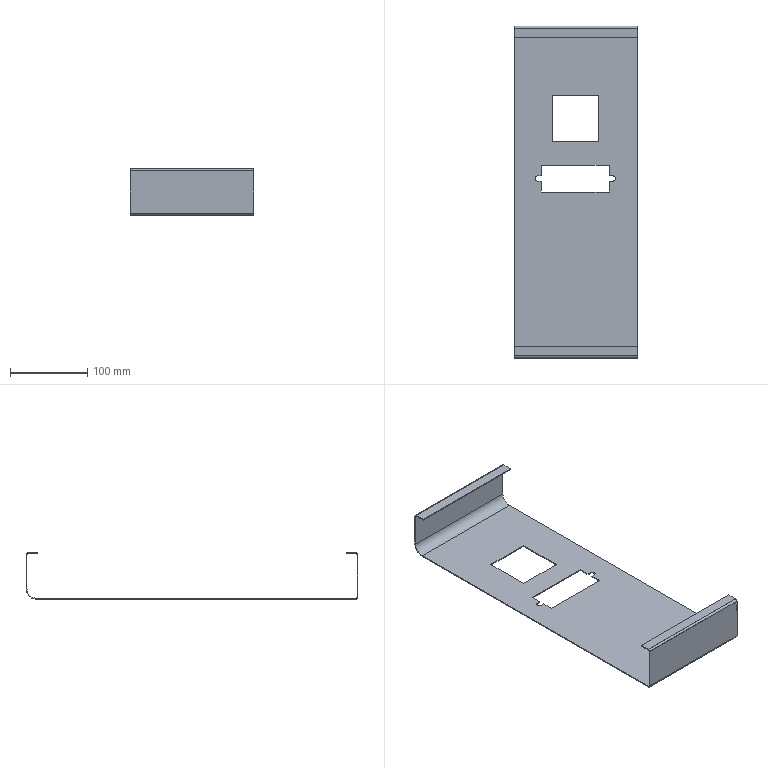Part | SolidWorks | features FlatPattern 1, ICE 1, SMBaseFlange 1, SheetMetal 1 | 1 solid | 55 faces | box 160 x 430 x 60 mm | volume 100743 mm3 | plane 44 | cylinder 11 | commonest cylinder face diameters 3 x3 5.4 x3 7 x3 24 x1 26.4 x1
STEP:
#1=CARTESIAN_POINT('',(-49.5,21.,1.2));
#2=VERTEX_POINT('',#1);
#3=CARTESIAN_POINT('',(-53.,17.5,1.2));
#4=VERTEX_POINT('',#3);
#5=CARTESIAN_POINT('',(-49.5,17.5,1.2));
#6=DIRECTION('',(0.,0.,1.));
#7=DIRECTION('',(0.,1.,0.));
#8=AXIS2_PLACEMENT_3D('',#5,#6,#7);
#9=CIRCLE('',#8,3.5);
#10=EDGE_CURVE('',#2,#4,#9,.T.);
#11=ORIENTED_EDGE('',*,*,#10,.T.);
#12=CARTESIAN_POINT('',(-53.,17.5,0.));
#13=VERTEX_POINT('',#12);
#14=CARTESIAN_POINT('',(-53.,17.5,60.001));
#15=DIRECTION('',(0.,0.,-1.));
#16=VECTOR('',#15,1000.);
#17=LINE('',#14,#16);
#18=EDGE_CURVE('',#4,#13,#17,.T.);
#19=ORIENTED_EDGE('',*,*,#18,.T.);
#20=CARTESIAN_POINT('',(-49.5,21.,0.));
#21=VERTEX_POINT('',#20);
#22=CARTESIAN_POINT('',(-49.5,17.5,0.));
#23=DIRECTION('',(0.,0.,-1.));
#24=DIRECTION('',(-1.,0.,0.));
#25=AXIS2_PLACEMENT_3D('',#22,#23,#24);
#26=CIRCLE('',#25,3.5);
#27=EDGE_CURVE('',#13,#21,#26,.T.);
#28=ORIENTED_EDGE('',*,*,#27,.T.);
#29=CARTESIAN_POINT('',(-49.5,21.,60.001));
#30=DIRECTION('',(0.,0.,-1.));
#31=VECTOR('',#30,1000.);
#32=LINE('',#29,#31);
#33=EDGE_CURVE('',#2,#21,#32,.T.);
#34=ORIENTED_EDGE('',*,*,#33,.F.);
#35=EDGE_LOOP('',(#11,#19,#28,#34));
#36=FACE_OUTER_BOUND('',#35,.T.);
#37=CARTESIAN_POINT('',(-49.5,17.5,60.001));
#38=DIRECTION('',(0.,0.,-1.));
#39=DIRECTION('',(-1.,0.,0.));
#40=AXIS2_PLACEMENT_3D('',#37,#38,#39);
#41=CYLINDRICAL_SURFACE('',#40,3.5);
#42=ADVANCED_FACE('',(#36),#41,.F.);
#43=CARTESIAN_POINT('',(80.,201.8,0.));
#44=VERTEX_POINT('',#43);
#45=CARTESIAN_POINT('',(80.,201.8,1.2));
#46=VERTEX_POINT('',#45);
#47=CARTESIAN_POINT('',(80.,201.8,0.));
#48=DIRECTION('',(0.,0.,1.));
#49=VECTOR('',#48,1000.);
#50=LINE('',#47,#49);
#51=EDGE_CURVE('',#44,#46,#50,.T.);
#52=ORIENTED_EDGE('',*,*,#51,.F.);
#53=CARTESIAN_POINT('',(80.,215.,13.2));
#54=VERTEX_POINT('',#53);
#55=CARTESIAN_POINT('',(80.,201.8,13.2));
#56=DIRECTION('',(-1.,0.,0.));
#57=DIRECTION('',(0.,0.,-1.));
#58=AXIS2_PLACEMENT_3D('',#55,#56,#57);
#59=CIRCLE('',#58,13.2);
#60=EDGE_CURVE('',#54,#44,#59,.T.);
#61=ORIENTED_EDGE('',*,*,#60,.F.);
#62=CARTESIAN_POINT('',(80.,213.8,13.2));
#63=VERTEX_POINT('',#62);
#64=CARTESIAN_POINT('',(80.,213.8,13.2));
#65=DIRECTION('',(0.,1.,0.));
#66=VECTOR('',#65,1000.);
#67=LINE('',#64,#66);
#68=EDGE_CURVE('',#63,#54,#67,.T.);
#69=ORIENTED_EDGE('',*,*,#68,.F.);
#70=CARTESIAN_POINT('',(80.,201.8,13.2));
#71=DIRECTION('',(-1.,0.,0.));
#72=DIRECTION('',(0.,0.,-1.));
#73=AXIS2_PLACEMENT_3D('',#70,#71,#72);
#74=CIRCLE('',#73,12.);
#75=EDGE_CURVE('',#63,#46,#74,.T.);
#76=ORIENTED_EDGE('',*,*,#75,.T.);
#77=EDGE_LOOP('',(#52,#61,#69,#76));
#78=FACE_OUTER_BOUND('',#77,.T.);
#79=CARTESIAN_POINT('',(80.,201.8,0.));
#80=DIRECTION('',(1.,0.,0.));
#81=DIRECTION('',(0.,0.,-1.));
#82=AXIS2_PLACEMENT_3D('',#79,#80,#81);
#83=PLANE('',#82);
#84=ADVANCED_FACE('',(#78),#83,.T.);
#85=CARTESIAN_POINT('',(80.,-212.3,0.));
#86=VERTEX_POINT('',#85);
#87=CARTESIAN_POINT('',(80.,0.,0.));
#88=DIRECTION('',(0.,-1.,0.));
#89=VECTOR('',#88,1000.);
#90=LINE('',#87,#89);
#91=EDGE_CURVE('',#44,#86,#90,.T.);
#92=ORIENTED_EDGE('',*,*,#91,.F.);
#93=ORIENTED_EDGE('',*,*,#51,.T.);
#94=CARTESIAN_POINT('',(80.,-212.3,1.2));
#95=VERTEX_POINT('',#94);
#96=CARTESIAN_POINT('',(80.,0.,1.2));
#97=DIRECTION('',(0.,-1.,0.));
#98=VECTOR('',#97,1000.);
#99=LINE('',#96,#98);
#100=EDGE_CURVE('',#46,#95,#99,.T.);
#101=ORIENTED_EDGE('',*,*,#100,.T.);
#102=CARTESIAN_POINT('',(80.,-212.3,1.2));
#103=DIRECTION('',(0.,0.,-1.));
#104=VECTOR('',#103,1000.);
#105=LINE('',#102,#104);
#106=EDGE_CURVE('',#95,#86,#105,.T.);
#107=ORIENTED_EDGE('',*,*,#106,.T.);
#108=EDGE_LOOP('',(#92,#93,#101,#107));
#109=FACE_OUTER_BOUND('',#108,.T.);
#110=CARTESIAN_POINT('',(80.,213.8,13.2));
#111=DIRECTION('',(1.,0.,0.));
#112=DIRECTION('',(0.,0.,-1.));
#113=AXIS2_PLACEMENT_3D('',#110,#111,#112);
#114=PLANE('',#113);
#115=ADVANCED_FACE('',(#109),#114,.T.);
#116=CARTESIAN_POINT('',(-80.,215.,13.2));
#117=VERTEX_POINT('',#116);
#118=CARTESIAN_POINT('',(-80.,213.8,13.2));
#119=VERTEX_POINT('',#118);
#120=CARTESIAN_POINT('',(-80.,215.,13.2));
#121=DIRECTION('',(0.,-1.,0.));
#122=VECTOR('',#121,1000.);
#123=LINE('',#120,#122);
#124=EDGE_CURVE('',#117,#119,#123,.T.);
#125=ORIENTED_EDGE('',*,*,#124,.F.);
#126=CARTESIAN_POINT('',(-80.,201.8,0.));
#127=VERTEX_POINT('',#126);
#128=CARTESIAN_POINT('',(-80.,201.8,13.2));
#129=DIRECTION('',(-1.,0.,0.));
#130=DIRECTION('',(0.,0.,-1.));
#131=AXIS2_PLACEMENT_3D('',#128,#129,#130);
#132=CIRCLE('',#131,13.2);
#133=EDGE_CURVE('',#117,#127,#132,.T.);
#134=ORIENTED_EDGE('',*,*,#133,.T.);
#135=CARTESIAN_POINT('',(-80.,201.8,1.2));
#136=VERTEX_POINT('',#135);
#137=CARTESIAN_POINT('',(-80.,201.8,1.2));
#138=DIRECTION('',(0.,0.,-1.));
#139=VECTOR('',#138,1000.);
#140=LINE('',#137,#139);
#141=EDGE_CURVE('',#136,#127,#140,.T.);
#142=ORIENTED_EDGE('',*,*,#141,.F.);
#143=CARTESIAN_POINT('',(-80.,201.8,13.2));
#144=DIRECTION('',(-1.,0.,0.));
#145=DIRECTION('',(0.,0.,-1.));
#146=AXIS2_PLACEMENT_3D('',#143,#144,#145);
#147=CIRCLE('',#146,12.);
#148=EDGE_CURVE('',#119,#136,#147,.T.);
#149=ORIENTED_EDGE('',*,*,#148,.F.);
#150=EDGE_LOOP('',(#125,#134,#142,#149));
#151=FACE_OUTER_BOUND('',#150,.T.);
#152=CARTESIAN_POINT('',(-80.,215.,13.2));
#153=DIRECTION('',(-1.,0.,0.));
#154=DIRECTION('',(0.,0.,1.));
#155=AXIS2_PLACEMENT_3D('',#152,#153,#154);
#156=PLANE('',#155);
#157=ADVANCED_FACE('',(#151),#156,.T.);
#158=CARTESIAN_POINT('',(-80.,215.,57.3));
#159=VERTEX_POINT('',#158);
#160=CARTESIAN_POINT('',(-80.,215.,13.2));
#161=DIRECTION('',(0.,0.,-1.));
#162=VECTOR('',#161,1000.);
#163=LINE('',#160,#162);
#164=EDGE_CURVE('',#159,#117,#163,.T.);
#165=ORIENTED_EDGE('',*,*,#164,.T.);
#166=ORIENTED_EDGE('',*,*,#124,.T.);
#167=CARTESIAN_POINT('',(-80.,213.8,57.3));
#168=VERTEX_POINT('',#167);
#169=CARTESIAN_POINT('',(-80.,213.8,13.2));
#170=DIRECTION('',(0.,0.,-1.));
#171=VECTOR('',#170,1000.);
#172=LINE('',#169,#171);
#173=EDGE_CURVE('',#168,#119,#172,.T.);
#174=ORIENTED_EDGE('',*,*,#173,.F.);
#175=CARTESIAN_POINT('',(-80.,213.8,57.3));
#176=DIRECTION('',(0.,1.,0.));
#177=VECTOR('',#176,1000.);
#178=LINE('',#175,#177);
#179=EDGE_CURVE('',#168,#159,#178,.T.);
#180=ORIENTED_EDGE('',*,*,#179,.T.);
#181=EDGE_LOOP('',(#165,#166,#174,#180));
#182=FACE_OUTER_BOUND('',#181,.T.);
#183=CARTESIAN_POINT('',(-80.,201.8,1.2));
#184=DIRECTION('',(-1.,0.,0.));
#185=DIRECTION('',(0.,0.,1.));
#186=AXIS2_PLACEMENT_3D('',#183,#184,#185);
#187=PLANE('',#186);
#188=ADVANCED_FACE('',(#182),#187,.T.);
#189=CARTESIAN_POINT('',(80.,215.,57.3));
#190=VERTEX_POINT('',#189);
#191=CARTESIAN_POINT('',(80.,213.8,57.3));
#192=VERTEX_POINT('',#191);
#193=CARTESIAN_POINT('',(80.,215.,57.3));
#194=DIRECTION('',(0.,-1.,0.));
#195=VECTOR('',#194,1000.);
#196=LINE('',#193,#195);
#197=EDGE_CURVE('',#190,#192,#196,.T.);
#198=ORIENTED_EDGE('',*,*,#197,.F.);
#199=CARTESIAN_POINT('',(80.,212.3,60.));
#200=VERTEX_POINT('',#199);
#201=CARTESIAN_POINT('',(80.,212.3,57.3));
#202=DIRECTION('',(-1.,0.,0.));
#203=DIRECTION('',(0.,0.,-1.));
#204=AXIS2_PLACEMENT_3D('',#201,#202,#203);
#205=CIRCLE('',#204,2.7);
#206=EDGE_CURVE('',#200,#190,#205,.T.);
#207=ORIENTED_EDGE('',*,*,#206,.F.);
#208=CARTESIAN_POINT('',(80.,212.3,58.8));
#209=VERTEX_POINT('',#208);
#210=CARTESIAN_POINT('',(80.,212.3,58.8));
#211=DIRECTION('',(0.,0.,1.));
#212=VECTOR('',#211,1000.);
#213=LINE('',#210,#212);
#214=EDGE_CURVE('',#209,#200,#213,.T.);
#215=ORIENTED_EDGE('',*,*,#214,.F.);
#216=CARTESIAN_POINT('',(80.,212.3,57.3));
#217=DIRECTION('',(-1.,0.,0.));
#218=DIRECTION('',(0.,0.,-1.));
#219=AXIS2_PLACEMENT_3D('',#216,#217,#218);
#220=CIRCLE('',#219,1.5);
#221=EDGE_CURVE('',#209,#192,#220,.T.);
#222=ORIENTED_EDGE('',*,*,#221,.T.);
#223=EDGE_LOOP('',(#198,#207,#215,#222));
#224=FACE_OUTER_BOUND('',#223,.T.);
#225=CARTESIAN_POINT('',(80.,215.,57.3));
#226=DIRECTION('',(1.,0.,0.));
#227=DIRECTION('',(0.,0.,-1.));
#228=AXIS2_PLACEMENT_3D('',#225,#226,#227);
#229=PLANE('',#228);
#230=ADVANCED_FACE('',(#224),#229,.T.);
#231=CARTESIAN_POINT('',(80.,215.,13.2));
#232=DIRECTION('',(0.,0.,-1.));
#233=VECTOR('',#232,1000.);
#234=LINE('',#231,#233);
#235=EDGE_CURVE('',#190,#54,#234,.T.);
#236=ORIENTED_EDGE('',*,*,#235,.F.);
#237=ORIENTED_EDGE('',*,*,#197,.T.);
#238=CARTESIAN_POINT('',(80.,213.8,13.2));
#239=DIRECTION('',(0.,0.,-1.));
#240=VECTOR('',#239,1000.);
#241=LINE('',#238,#240);
#242=EDGE_CURVE('',#192,#63,#241,.T.);
#243=ORIENTED_EDGE('',*,*,#242,.T.);
#244=ORIENTED_EDGE('',*,*,#68,.T.);
#245=EDGE_LOOP('',(#236,#237,#243,#244));
#246=FACE_OUTER_BOUND('',#245,.T.);
#247=CARTESIAN_POINT('',(80.,212.3,58.8));
#248=DIRECTION('',(1.,0.,0.));
#249=DIRECTION('',(0.,0.,-1.));
#250=AXIS2_PLACEMENT_3D('',#247,#248,#249);
#251=PLANE('',#250);
#252=ADVANCED_FACE('',(#246),#251,.T.);
#253=CARTESIAN_POINT('',(-80.,212.3,60.));
#254=VERTEX_POINT('',#253);
#255=CARTESIAN_POINT('',(-80.,212.3,58.8));
#256=VERTEX_POINT('',#255);
#257=CARTESIAN_POINT('',(-80.,212.3,60.));
#258=DIRECTION('',(0.,0.,-1.));
#259=VECTOR('',#258,1000.);
#260=LINE('',#257,#259);
#261=EDGE_CURVE('',#254,#256,#260,.T.);
#262=ORIENTED_EDGE('',*,*,#261,.F.);
#263=CARTESIAN_POINT('',(-80.,212.3,57.3));
#264=DIRECTION('',(-1.,0.,0.));
#265=DIRECTION('',(0.,0.,-1.));
#266=AXIS2_PLACEMENT_3D('',#263,#264,#265);
#267=CIRCLE('',#266,2.7);
#268=EDGE_CURVE('',#254,#159,#267,.T.);
#269=ORIENTED_EDGE('',*,*,#268,.T.);
#270=ORIENTED_EDGE('',*,*,#179,.F.);
#271=CARTESIAN_POINT('',(-80.,212.3,57.3));
#272=DIRECTION('',(-1.,0.,0.));
#273=DIRECTION('',(0.,0.,-1.));
#274=AXIS2_PLACEMENT_3D('',#271,#272,#273);
#275=CIRCLE('',#274,1.5);
#276=EDGE_CURVE('',#256,#168,#275,.T.);
#277=ORIENTED_EDGE('',*,*,#276,.F.);
#278=EDGE_LOOP('',(#262,#269,#270,#277));
#279=FACE_OUTER_BOUND('',#278,.T.);
#280=CARTESIAN_POINT('',(-80.,212.3,60.));
#281=DIRECTION('',(-1.,0.,0.));
#282=DIRECTION('',(0.,0.,1.));
#283=AXIS2_PLACEMENT_3D('',#280,#281,#282);
#284=PLANE('',#283);
#285=ADVANCED_FACE('',(#279),#284,.T.);
#286=CARTESIAN_POINT('',(-80.,200.,60.));
#287=VERTEX_POINT('',#286);
#288=CARTESIAN_POINT('',(-80.,215.,60.));
#289=DIRECTION('',(0.,1.,0.));
#290=VECTOR('',#289,1000.);
#291=LINE('',#288,#290);
#292=EDGE_CURVE('',#287,#254,#291,.T.);
#293=ORIENTED_EDGE('',*,*,#292,.T.);
#294=ORIENTED_EDGE('',*,*,#261,.T.);
#295=CARTESIAN_POINT('',(-80.,200.,58.8));
#296=VERTEX_POINT('',#295);
#297=CARTESIAN_POINT('',(-80.,215.,58.8));
#298=DIRECTION('',(0.,1.,0.));
#299=VECTOR('',#298,1000.);
#300=LINE('',#297,#299);
#301=EDGE_CURVE('',#296,#256,#300,.T.);
#302=ORIENTED_EDGE('',*,*,#301,.F.);
#303=CARTESIAN_POINT('',(-80.,200.,58.8));
#304=DIRECTION('',(0.,0.,1.));
#305=VECTOR('',#304,1000.);
#306=LINE('',#303,#305);
#307=EDGE_CURVE('',#296,#287,#306,.T.);
#308=ORIENTED_EDGE('',*,*,#307,.T.);
#309=EDGE_LOOP('',(#293,#294,#302,#308));
#310=FACE_OUTER_BOUND('',#309,.T.);
#311=CARTESIAN_POINT('',(-80.,213.8,57.3));
#312=DIRECTION('',(-1.,0.,0.));
#313=DIRECTION('',(0.,0.,1.));
#314=AXIS2_PLACEMENT_3D('',#311,#312,#313);
#315=PLANE('',#314);
#316=ADVANCED_FACE('',(#310),#315,.T.);
#317=CARTESIAN_POINT('',(80.,-215.,2.7));
#318=VERTEX_POINT('',#317);
#319=CARTESIAN_POINT('',(80.,-213.8,2.7));
#320=VERTEX_POINT('',#319);
#321=CARTESIAN_POINT('',(80.,-215.,2.7));
#322=DIRECTION('',(0.,1.,0.));
#323=VECTOR('',#322,1000.);
#324=LINE('',#321,#323);
#325=EDGE_CURVE('',#318,#320,#324,.T.);
#326=ORIENTED_EDGE('',*,*,#325,.F.);
#327=CARTESIAN_POINT('',(80.,-212.3,2.7));
#328=DIRECTION('',(-1.,0.,0.));
#329=DIRECTION('',(0.,0.,-1.));
#330=AXIS2_PLACEMENT_3D('',#327,#328,#329);
#331=CIRCLE('',#330,2.7);
#332=EDGE_CURVE('',#86,#318,#331,.T.);
#333=ORIENTED_EDGE('',*,*,#332,.F.);
#334=ORIENTED_EDGE('',*,*,#106,.F.);
#335=CARTESIAN_POINT('',(80.,-212.3,2.7));
#336=DIRECTION('',(-1.,0.,0.));
#337=DIRECTION('',(0.,0.,-1.));
#338=AXIS2_PLACEMENT_3D('',#335,#336,#337);
#339=CIRCLE('',#338,1.5);
#340=EDGE_CURVE('',#95,#320,#339,.T.);
#341=ORIENTED_EDGE('',*,*,#340,.T.);
#342=EDGE_LOOP('',(#326,#333,#334,#341));
#343=FACE_OUTER_BOUND('',#342,.T.);
#344=CARTESIAN_POINT('',(80.,-215.,2.7));
#345=DIRECTION('',(1.,0.,0.));
#346=DIRECTION('',(0.,0.,-1.));
#347=AXIS2_PLACEMENT_3D('',#344,#345,#346);
#348=PLANE('',#347);
#349=ADVANCED_FACE('',(#343),#348,.T.);
#350=CARTESIAN_POINT('',(80.,-215.,57.3));
#351=VERTEX_POINT('',#350);
#352=CARTESIAN_POINT('',(80.,-215.,0.));
#353=DIRECTION('',(0.,0.,1.));
#354=VECTOR('',#353,1000.);
#355=LINE('',#352,#354);
#356=EDGE_CURVE('',#318,#351,#355,.T.);
#357=ORIENTED_EDGE('',*,*,#356,.F.);
#358=ORIENTED_EDGE('',*,*,#325,.T.);
#359=CARTESIAN_POINT('',(80.,-213.8,57.3));
#360=VERTEX_POINT('',#359);
#361=CARTESIAN_POINT('',(80.,-213.8,0.));
#362=DIRECTION('',(0.,0.,1.));
#363=VECTOR('',#362,1000.);
#364=LINE('',#361,#363);
#365=EDGE_CURVE('',#320,#360,#364,.T.);
#366=ORIENTED_EDGE('',*,*,#365,.T.);
#367=CARTESIAN_POINT('',(80.,-213.8,57.3));
#368=DIRECTION('',(0.,-1.,0.));
#369=VECTOR('',#368,1000.);
#370=LINE('',#367,#369);
#371=EDGE_CURVE('',#360,#351,#370,.T.);
#372=ORIENTED_EDGE('',*,*,#371,.T.);
#373=EDGE_LOOP('',(#357,#358,#366,#372));
#374=FACE_OUTER_BOUND('',#373,.T.);
#375=CARTESIAN_POINT('',(80.,-212.3,1.2));
#376=DIRECTION('',(1.,0.,0.));
#377=DIRECTION('',(0.,0.,-1.));
#378=AXIS2_PLACEMENT_3D('',#375,#376,#377);
#379=PLANE('',#378);
#380=ADVANCED_FACE('',(#374),#379,.T.);
#381=CARTESIAN_POINT('',(-80.,-212.3,0.));
#382=VERTEX_POINT('',#381);
#383=CARTESIAN_POINT('',(-80.,-212.3,1.2));
#384=VERTEX_POINT('',#383);
#385=CARTESIAN_POINT('',(-80.,-212.3,0.));
#386=DIRECTION('',(0.,0.,1.));
#387=VECTOR('',#386,1000.);
#388=LINE('',#385,#387);
#389=EDGE_CURVE('',#382,#384,#388,.T.);
#390=ORIENTED_EDGE('',*,*,#389,.F.);
#391=CARTESIAN_POINT('',(-80.,-215.,2.7));
#392=VERTEX_POINT('',#391);
#393=CARTESIAN_POINT('',(-80.,-212.3,2.7));
#394=DIRECTION('',(-1.,0.,0.));
#395=DIRECTION('',(0.,0.,-1.));
#396=AXIS2_PLACEMENT_3D('',#393,#394,#395);
#397=CIRCLE('',#396,2.7);
#398=EDGE_CURVE('',#382,#392,#397,.T.);
#399=ORIENTED_EDGE('',*,*,#398,.T.);
#400=CARTESIAN_POINT('',(-80.,-213.8,2.7));
#401=VERTEX_POINT('',#400);
#402=CARTESIAN_POINT('',(-80.,-213.8,2.7));
#403=DIRECTION('',(0.,-1.,0.));
#404=VECTOR('',#403,1000.);
#405=LINE('',#402,#404);
#406=EDGE_CURVE('',#401,#392,#405,.T.);
#407=ORIENTED_EDGE('',*,*,#406,.F.);
#408=CARTESIAN_POINT('',(-80.,-212.3,2.7));
#409=DIRECTION('',(-1.,0.,0.));
#410=DIRECTION('',(0.,0.,-1.));
#411=AXIS2_PLACEMENT_3D('',#408,#409,#410);
#412=CIRCLE('',#411,1.5);
#413=EDGE_CURVE('',#384,#401,#412,.T.);
#414=ORIENTED_EDGE('',*,*,#413,.F.);
#415=EDGE_LOOP('',(#390,#399,#407,#414));
#416=FACE_OUTER_BOUND('',#415,.T.);
#417=CARTESIAN_POINT('',(-80.,-212.3,0.));
#418=DIRECTION('',(-1.,0.,0.));
#419=DIRECTION('',(0.,0.,1.));
#420=AXIS2_PLACEMENT_3D('',#417,#418,#419);
#421=PLANE('',#420);
#422=ADVANCED_FACE('',(#416),#421,.T.);
#423=CARTESIAN_POINT('',(-80.,0.,0.));
#424=DIRECTION('',(0.,-1.,0.));
#425=VECTOR('',#424,1000.);
#426=LINE('',#423,#425);
#427=EDGE_CURVE('',#127,#382,#426,.T.);
#428=ORIENTED_EDGE('',*,*,#427,.T.);
#429=ORIENTED_EDGE('',*,*,#389,.T.);
#430=CARTESIAN_POINT('',(-80.,0.,1.2));
#431=DIRECTION('',(0.,-1.,0.));
#432=VECTOR('',#431,1000.);
#433=LINE('',#430,#432);
#434=EDGE_CURVE('',#136,#384,#433,.T.);
#435=ORIENTED_EDGE('',*,*,#434,.F.);
#436=ORIENTED_EDGE('',*,*,#141,.T.);
#437=EDGE_LOOP('',(#428,#429,#435,#436));
#438=FACE_OUTER_BOUND('',#437,.T.);
#439=CARTESIAN_POINT('',(-80.,-213.8,2.7));
#440=DIRECTION('',(-1.,0.,0.));
#441=DIRECTION('',(0.,0.,1.));
#442=AXIS2_PLACEMENT_3D('',#439,#440,#441);
#443=PLANE('',#442);
#444=ADVANCED_FACE('',(#438),#443,.T.);
#445=CARTESIAN_POINT('',(80.,-212.3,60.));
#446=VERTEX_POINT('',#445);
#447=CARTESIAN_POINT('',(80.,-212.3,58.8));
#448=VERTEX_POINT('',#447);
#449=CARTESIAN_POINT('',(80.,-212.3,60.));
#450=DIRECTION('',(0.,0.,-1.));
#451=VECTOR('',#450,1000.);
#452=LINE('',#449,#451);
#453=EDGE_CURVE('',#446,#448,#452,.T.);
#454=ORIENTED_EDGE('',*,*,#453,.F.);
#455=CARTESIAN_POINT('',(80.,-212.3,57.3));
#456=DIRECTION('',(-1.,0.,0.));
#457=DIRECTION('',(0.,0.,-1.));
#458=AXIS2_PLACEMENT_3D('',#455,#456,#457);
#459=CIRCLE('',#458,2.7);
#460=EDGE_CURVE('',#351,#446,#459,.T.);
#461=ORIENTED_EDGE('',*,*,#460,.F.);
#462=ORIENTED_EDGE('',*,*,#371,.F.);
#463=CARTESIAN_POINT('',(80.,-212.3,57.3));
#464=DIRECTION('',(-1.,0.,0.));
#465=DIRECTION('',(0.,0.,-1.));
#466=AXIS2_PLACEMENT_3D('',#463,#464,#465);
#467=CIRCLE('',#466,1.5);
#468=EDGE_CURVE('',#360,#448,#467,.T.);
#469=ORIENTED_EDGE('',*,*,#468,.T.);
#470=EDGE_LOOP('',(#454,#461,#462,#469));
#471=FACE_OUTER_BOUND('',#470,.T.);
#472=CARTESIAN_POINT('',(80.,-212.3,60.));
#473=DIRECTION('',(1.,0.,0.));
#474=DIRECTION('',(0.,0.,-1.));
#475=AXIS2_PLACEMENT_3D('',#472,#473,#474);
#476=PLANE('',#475);
#477=ADVANCED_FACE('',(#471),#476,.T.);
#478=CARTESIAN_POINT('',(80.,-200.,60.));
#479=VERTEX_POINT('',#478);
#480=CARTESIAN_POINT('',(80.,-215.,60.));
#481=DIRECTION('',(0.,1.,0.));
#482=VECTOR('',#481,1000.);
#483=LINE('',#480,#482);
#484=EDGE_CURVE('',#446,#479,#483,.T.);
#485=ORIENTED_EDGE('',*,*,#484,.F.);
#486=ORIENTED_EDGE('',*,*,#453,.T.);
#487=CARTESIAN_POINT('',(80.,-200.,58.8));
#488=VERTEX_POINT('',#487);
#489=CARTESIAN_POINT('',(80.,-215.,58.8));
#490=DIRECTION('',(0.,1.,0.));
#491=VECTOR('',#490,1000.);
#492=LINE('',#489,#491);
#493=EDGE_CURVE('',#448,#488,#492,.T.);
#494=ORIENTED_EDGE('',*,*,#493,.T.);
#495=CARTESIAN_POINT('',(80.,-200.,60.));
#496=DIRECTION('',(0.,0.,-1.));
#497=VECTOR('',#496,1000.);
#498=LINE('',#495,#497);
#499=EDGE_CURVE('',#479,#488,#498,.T.);
#500=ORIENTED_EDGE('',*,*,#499,.F.);
#501=EDGE_LOOP('',(#485,#486,#494,#500));
#502=FACE_OUTER_BOUND('',#501,.T.);
#503=CARTESIAN_POINT('',(80.,-213.8,57.3));
#504=DIRECTION('',(1.,0.,0.));
#505=DIRECTION('',(0.,0.,-1.));
#506=AXIS2_PLACEMENT_3D('',#503,#504,#505);
#507=PLANE('',#506);
#508=ADVANCED_FACE('',(#502),#507,.T.);
#509=CARTESIAN_POINT('',(-80.,-215.,57.3));
#510=VERTEX_POINT('',#509);
#511=CARTESIAN_POINT('',(-80.,-213.8,57.3));
#512=VERTEX_POINT('',#511);
#513=CARTESIAN_POINT('',(-80.,-215.,57.3));
#514=DIRECTION('',(0.,1.,0.));
#515=VECTOR('',#514,1000.);
#516=LINE('',#513,#515);
#517=EDGE_CURVE('',#510,#512,#516,.T.);
#518=ORIENTED_EDGE('',*,*,#517,.F.);
#519=CARTESIAN_POINT('',(-80.,-212.3,60.));
#520=VERTEX_POINT('',#519);
#521=CARTESIAN_POINT('',(-80.,-212.3,57.3));
#522=DIRECTION('',(-1.,0.,0.));
#523=DIRECTION('',(0.,0.,-1.));
#524=AXIS2_PLACEMENT_3D('',#521,#522,#523);
#525=CIRCLE('',#524,2.7);
#526=EDGE_CURVE('',#510,#520,#525,.T.);
#527=ORIENTED_EDGE('',*,*,#526,.T.);
#528=CARTESIAN_POINT('',(-80.,-212.3,58.8));
#529=VERTEX_POINT('',#528);
#530=CARTESIAN_POINT('',(-80.,-212.3,58.8));
#531=DIRECTION('',(0.,0.,1.));
#532=VECTOR('',#531,1000.);
#533=LINE('',#530,#532);
#534=EDGE_CURVE('',#529,#520,#533,.T.);
#535=ORIENTED_EDGE('',*,*,#534,.F.);
#536=CARTESIAN_POINT('',(-80.,-212.3,57.3));
#537=DIRECTION('',(-1.,0.,0.));
#538=DIRECTION('',(0.,0.,-1.));
#539=AXIS2_PLACEMENT_3D('',#536,#537,#538);
#540=CIRCLE('',#539,1.5);
#541=EDGE_CURVE('',#512,#529,#540,.T.);
#542=ORIENTED_EDGE('',*,*,#541,.F.);
#543=EDGE_LOOP('',(#518,#527,#535,#542));
#544=FACE_OUTER_BOUND('',#543,.T.);
#545=CARTESIAN_POINT('',(-80.,-215.,57.3));
#546=DIRECTION('',(-1.,0.,0.));
#547=DIRECTION('',(0.,0.,1.));
#548=AXIS2_PLACEMENT_3D('',#545,#546,#547);
#549=PLANE('',#548);
#550=ADVANCED_FACE('',(#544),#549,.T.);
#551=CARTESIAN_POINT('',(-80.,-215.,0.));
#552=DIRECTION('',(0.,0.,1.));
#553=VECTOR('',#552,1000.);
#554=LINE('',#551,#553);
#555=EDGE_CURVE('',#392,#510,#554,.T.);
#556=ORIENTED_EDGE('',*,*,#555,.T.);
#557=ORIENTED_EDGE('',*,*,#517,.T.);
#558=CARTESIAN_POINT('',(-80.,-213.8,0.));
#559=DIRECTION('',(0.,0.,1.));
#560=VECTOR('',#559,1000.);
#561=LINE('',#558,#560);
#562=EDGE_CURVE('',#401,#512,#561,.T.);
#563=ORIENTED_EDGE('',*,*,#562,.F.);
#564=ORIENTED_EDGE('',*,*,#406,.T.);
#565=EDGE_LOOP('',(#556,#557,#563,#564));
#566=FACE_OUTER_BOUND('',#565,.T.);
#567=CARTESIAN_POINT('',(-80.,-212.3,58.8));
#568=DIRECTION('',(-1.,0.,0.));
#569=DIRECTION('',(0.,0.,1.));
#570=AXIS2_PLACEMENT_3D('',#567,#568,#569);
#571=PLANE('',#570);
#572=ADVANCED_FACE('',(#566),#571,.T.);
#573=CARTESIAN_POINT('',(-80.,-200.,58.8));
#574=VERTEX_POINT('',#573);
#575=CARTESIAN_POINT('',(-80.,-215.,58.8));
#576=DIRECTION('',(0.,1.,0.));
#577=VECTOR('',#576,1000.);
#578=LINE('',#575,#577);
#579=EDGE_CURVE('',#529,#574,#578,.T.);
#580=ORIENTED_EDGE('',*,*,#579,.T.);
#581=CARTESIAN_POINT('',(80.,-200.,58.8));
#582=DIRECTION('',(-1.,0.,0.));
#583=VECTOR('',#582,1000.);
#584=LINE('',#581,#583);
#585=EDGE_CURVE('',#488,#574,#584,.T.);
#586=ORIENTED_EDGE('',*,*,#585,.F.);
#587=ORIENTED_EDGE('',*,*,#493,.F.);
#588=CARTESIAN_POINT('',(80.,-212.3,58.8));
#589=DIRECTION('',(-1.,0.,0.));
#590=VECTOR('',#589,1000.);
#591=LINE('',#588,#590);
#592=EDGE_CURVE('',#448,#529,#591,.T.);
#593=ORIENTED_EDGE('',*,*,#592,.T.);
#594=EDGE_LOOP('',(#580,#586,#587,#593));
#595=FACE_OUTER_BOUND('',#594,.T.);
#596=CARTESIAN_POINT('',(80.,-215.,58.8));
#597=DIRECTION('',(0.,0.,1.));
#598=DIRECTION('',(1.,0.,0.));
#599=AXIS2_PLACEMENT_3D('',#596,#597,#598);
#600=PLANE('',#599);
#601=ADVANCED_FACE('',(#595),#600,.F.);
#602=CARTESIAN_POINT('',(-80.,-200.,60.));
#603=VERTEX_POINT('',#602);
#604=CARTESIAN_POINT('',(-80.,-200.,60.));
#605=DIRECTION('',(0.,0.,-1.));
#606=VECTOR('',#605,1000.);
#607=LINE('',#604,#606);
#608=EDGE_CURVE('',#603,#574,#607,.T.);
#609=ORIENTED_EDGE('',*,*,#608,.F.);
#610=CARTESIAN_POINT('',(80.,-200.,60.));
#611=DIRECTION('',(-1.,0.,0.));
#612=VECTOR('',#611,1000.);
#613=LINE('',#610,#612);
#614=EDGE_CURVE('',#479,#603,#613,.T.);
#615=ORIENTED_EDGE('',*,*,#614,.F.);
#616=ORIENTED_EDGE('',*,*,#499,.T.);
#617=ORIENTED_EDGE('',*,*,#585,.T.);
#618=EDGE_LOOP('',(#609,#615,#616,#617));
#619=FACE_OUTER_BOUND('',#618,.T.);
#620=CARTESIAN_POINT('',(80.,-200.,60.));
#621=DIRECTION('',(0.,1.,0.));
#622=DIRECTION('',(0.,0.,1.));
#623=AXIS2_PLACEMENT_3D('',#620,#621,#622);
#624=PLANE('',#623);
#625=ADVANCED_FACE('',(#619),#624,.T.);
#626=CARTESIAN_POINT('',(-80.,-215.,60.));
#627=DIRECTION('',(0.,1.,0.));
#628=VECTOR('',#627,1000.);
#629=LINE('',#626,#628);
#630=EDGE_CURVE('',#520,#603,#629,.T.);
#631=ORIENTED_EDGE('',*,*,#630,.F.);
#632=CARTESIAN_POINT('',(80.,-212.3,60.));
#633=DIRECTION('',(-1.,0.,0.));
#634=VECTOR('',#633,1000.);
#635=LINE('',#632,#634);
#636=EDGE_CURVE('',#446,#520,#635,.T.);
#637=ORIENTED_EDGE('',*,*,#636,.F.);
#638=ORIENTED_EDGE('',*,*,#484,.T.);
#639=ORIENTED_EDGE('',*,*,#614,.T.);
#640=EDGE_LOOP('',(#631,#637,#638,#639));
#641=FACE_OUTER_BOUND('',#640,.T.);
#642=CARTESIAN_POINT('',(80.,-215.,60.));
#643=DIRECTION('',(0.,0.,1.));
#644=DIRECTION('',(1.,0.,0.));
#645=AXIS2_PLACEMENT_3D('',#642,#643,#644);
#646=PLANE('',#645);
#647=ADVANCED_FACE('',(#641),#646,.T.);
#648=ORIENTED_EDGE('',*,*,#526,.F.);
#649=CARTESIAN_POINT('',(80.,-215.,57.3));
#650=DIRECTION('',(-1.,0.,0.));
#651=VECTOR('',#650,1000.);
#652=LINE('',#649,#651);
#653=EDGE_CURVE('',#351,#510,#652,.T.);
#654=ORIENTED_EDGE('',*,*,#653,.F.);
#655=ORIENTED_EDGE('',*,*,#460,.T.);
#656=ORIENTED_EDGE('',*,*,#636,.T.);
#657=EDGE_LOOP('',(#648,#654,#655,#656));
#658=FACE_OUTER_BOUND('',#657,.T.);
#659=CARTESIAN_POINT('',(80.,-212.3,57.3));
#660=DIRECTION('',(-1.,0.,0.));
#661=DIRECTION('',(0.,0.,1.));
#662=AXIS2_PLACEMENT_3D('',#659,#660,#661);
#663=CYLINDRICAL_SURFACE('',#662,2.7);
#664=ADVANCED_FACE('',(#658),#663,.T.);
#665=ORIENTED_EDGE('',*,*,#555,.F.);
#666=CARTESIAN_POINT('',(80.,-215.,2.7));
#667=DIRECTION('',(-1.,0.,0.));
#668=VECTOR('',#667,1000.);
#669=LINE('',#666,#668);
#670=EDGE_CURVE('',#318,#392,#669,.T.);
#671=ORIENTED_EDGE('',*,*,#670,.F.);
#672=ORIENTED_EDGE('',*,*,#356,.T.);
#673=ORIENTED_EDGE('',*,*,#653,.T.);
#674=EDGE_LOOP('',(#665,#671,#672,#673));
#675=FACE_OUTER_BOUND('',#674,.T.);
#676=CARTESIAN_POINT('',(80.,-215.,0.));
#677=DIRECTION('',(0.,-1.,0.));
#678=DIRECTION('',(0.,0.,-1.));
#679=AXIS2_PLACEMENT_3D('',#676,#677,#678);
#680=PLANE('',#679);
#681=ADVANCED_FACE('',(#675),#680,.T.);
#682=ORIENTED_EDGE('',*,*,#398,.F.);
#683=CARTESIAN_POINT('',(80.,-212.3,0.));
#684=DIRECTION('',(-1.,0.,0.));
#685=VECTOR('',#684,1000.);
#686=LINE('',#683,#685);
#687=EDGE_CURVE('',#86,#382,#686,.T.);
#688=ORIENTED_EDGE('',*,*,#687,.F.);
#689=ORIENTED_EDGE('',*,*,#332,.T.);
#690=ORIENTED_EDGE('',*,*,#670,.T.);
#691=EDGE_LOOP('',(#682,#688,#689,#690));
#692=FACE_OUTER_BOUND('',#691,.T.);
#693=CARTESIAN_POINT('',(80.,-212.3,2.7));
#694=DIRECTION('',(-1.,0.,0.));
#695=DIRECTION('',(0.,0.,1.));
#696=AXIS2_PLACEMENT_3D('',#693,#694,#695);
#697=CYLINDRICAL_SURFACE('',#696,2.7);
#698=ADVANCED_FACE('',(#692),#697,.T.);
#699=CARTESIAN_POINT('',(43.,35.,0.));
#700=VERTEX_POINT('',#699);
#701=CARTESIAN_POINT('',(43.,21.,0.));
#702=VERTEX_POINT('',#701);
#703=CARTESIAN_POINT('',(43.,35.,0.));
#704=DIRECTION('',(0.,-1.,0.));
#705=VECTOR('',#704,1000.);
#706=LINE('',#703,#705);
#707=EDGE_CURVE('',#700,#702,#706,.T.);
#708=ORIENTED_EDGE('',*,*,#707,.F.);
#709=CARTESIAN_POINT('',(-45.,35.,0.));
#710=VERTEX_POINT('',#709);
#711=CARTESIAN_POINT('',(43.,35.,0.));
#712=DIRECTION('',(1.,0.,0.));
#713=VECTOR('',#712,1000.);
#714=LINE('',#711,#713);
#715=EDGE_CURVE('',#710,#700,#714,.T.);
#716=ORIENTED_EDGE('',*,*,#715,.F.);
#717=CARTESIAN_POINT('',(-45.,21.,0.));
#718=VERTEX_POINT('',#717);
#719=CARTESIAN_POINT('',(-45.,35.,0.));
#720=DIRECTION('',(0.,1.,0.));
#721=VECTOR('',#720,1000.);
#722=LINE('',#719,#721);
#723=EDGE_CURVE('',#718,#710,#722,.T.);
#724=ORIENTED_EDGE('',*,*,#723,.F.);
#725=CARTESIAN_POINT('',(-49.5,21.,0.));
#726=DIRECTION('',(1.,0.,0.));
#727=VECTOR('',#726,1000.);
#728=LINE('',#725,#727);
#729=EDGE_CURVE('',#21,#718,#728,.T.);
#730=ORIENTED_EDGE('',*,*,#729,.F.);
#731=ORIENTED_EDGE('',*,*,#27,.F.);
#732=CARTESIAN_POINT('',(-49.5,14.,0.));
#733=VERTEX_POINT('',#732);
#734=CARTESIAN_POINT('',(-49.5,17.5,0.));
#735=DIRECTION('',(0.,0.,-1.));
#736=DIRECTION('',(-1.,0.,0.));
#737=AXIS2_PLACEMENT_3D('',#734,#735,#736);
#738=CIRCLE('',#737,3.5);
#739=EDGE_CURVE('',#733,#13,#738,.T.);
#740=ORIENTED_EDGE('',*,*,#739,.F.);
#741=CARTESIAN_POINT('',(-45.,14.,0.));
#742=VERTEX_POINT('',#741);
#743=CARTESIAN_POINT('',(-49.5,14.,0.));
#744=DIRECTION('',(-1.,0.,0.));
#745=VECTOR('',#744,1000.);
#746=LINE('',#743,#745);
#747=EDGE_CURVE('',#742,#733,#746,.T.);
#748=ORIENTED_EDGE('',*,*,#747,.F.);
#749=CARTESIAN_POINT('',(-45.,0.,0.));
#750=VERTEX_POINT('',#749);
#751=CARTESIAN_POINT('',(-45.,14.,0.));
#752=DIRECTION('',(0.,1.,0.));
#753=VECTOR('',#752,1000.);
#754=LINE('',#751,#753);
#755=EDGE_CURVE('',#750,#742,#754,.T.);
#756=ORIENTED_EDGE('',*,*,#755,.F.);
#757=CARTESIAN_POINT('',(43.,0.,0.));
#758=VERTEX_POINT('',#757);
#759=CARTESIAN_POINT('',(43.,0.,0.));
#760=DIRECTION('',(-1.,0.,0.));
#761=VECTOR('',#760,1000.);
#762=LINE('',#759,#761);
#763=EDGE_CURVE('',#758,#750,#762,.T.);
#764=ORIENTED_EDGE('',*,*,#763,.F.);
#765=CARTESIAN_POINT('',(43.,14.,0.));
#766=VERTEX_POINT('',#765);
#767=CARTESIAN_POINT('',(43.,14.,0.));
#768=DIRECTION('',(0.,-1.,0.));
#769=VECTOR('',#768,1000.);
#770=LINE('',#767,#769);
#771=EDGE_CURVE('',#766,#758,#770,.T.);
#772=ORIENTED_EDGE('',*,*,#771,.F.);
#773=CARTESIAN_POINT('',(47.5,14.,0.));
#774=VERTEX_POINT('',#773);
#775=CARTESIAN_POINT('',(47.5,14.,0.));
#776=DIRECTION('',(-1.,0.,0.));
#777=VECTOR('',#776,1000.);
#778=LINE('',#775,#777);
#779=EDGE_CURVE('',#774,#766,#778,.T.);
#780=ORIENTED_EDGE('',*,*,#779,.F.);
#781=CARTESIAN_POINT('',(47.5,21.,0.));
#782=VERTEX_POINT('',#781);
#783=CARTESIAN_POINT('',(47.5,17.5,0.));
#784=DIRECTION('',(0.,0.,-1.));
#785=DIRECTION('',(1.,0.,0.));
#786=AXIS2_PLACEMENT_3D('',#783,#784,#785);
#787=CIRCLE('',#786,3.5);
#788=EDGE_CURVE('',#782,#774,#787,.T.);
#789=ORIENTED_EDGE('',*,*,#788,.F.);
#790=CARTESIAN_POINT('',(47.5,21.,0.));
#791=DIRECTION('',(1.,0.,0.));
#792=VECTOR('',#791,1000.);
#793=LINE('',#790,#792);
#794=EDGE_CURVE('',#702,#782,#793,.T.);
#795=ORIENTED_EDGE('',*,*,#794,.F.);
#796=EDGE_LOOP('',(#708,#716,#724,#730,#731,#740,#748,#756,#764,#772,#780,#789,#795));
#797=FACE_BOUND('',#796,.T.);
#798=CARTESIAN_POINT('',(29.,125.,0.));
#799=VERTEX_POINT('',#798);
#800=CARTESIAN_POINT('',(29.,65.,0.));
#801=VERTEX_POINT('',#800);
#802=CARTESIAN_POINT('',(29.,125.,0.));
#803=DIRECTION('',(0.,-1.,0.));
#804=VECTOR('',#803,1000.);
#805=LINE('',#802,#804);
#806=EDGE_CURVE('',#799,#801,#805,.T.);
#807=ORIENTED_EDGE('',*,*,#806,.F.);
#808=CARTESIAN_POINT('',(-31.,125.,0.));
#809=VERTEX_POINT('',#808);
#810=CARTESIAN_POINT('',(29.,125.,0.));
#811=DIRECTION('',(1.,0.,0.));
#812=VECTOR('',#811,1000.);
#813=LINE('',#810,#812);
#814=EDGE_CURVE('',#809,#799,#813,.T.);
#815=ORIENTED_EDGE('',*,*,#814,.F.);
#816=CARTESIAN_POINT('',(-31.,65.,0.));
#817=VERTEX_POINT('',#816);
#818=CARTESIAN_POINT('',(-31.,125.,0.));
#819=DIRECTION('',(0.,1.,0.));
#820=VECTOR('',#819,1000.);
#821=LINE('',#818,#820);
#822=EDGE_CURVE('',#817,#809,#821,.T.);
#823=ORIENTED_EDGE('',*,*,#822,.F.);
#824=CARTESIAN_POINT('',(29.,65.,0.));
#825=DIRECTION('',(-1.,0.,0.));
#826=VECTOR('',#825,1000.);
#827=LINE('',#824,#826);
#828=EDGE_CURVE('',#801,#817,#827,.T.);
#829=ORIENTED_EDGE('',*,*,#828,.F.);
#830=EDGE_LOOP('',(#807,#815,#823,#829));
#831=FACE_BOUND('',#830,.T.);
#832=ORIENTED_EDGE('',*,*,#427,.F.);
#833=CARTESIAN_POINT('',(80.,201.8,0.));
#834=DIRECTION('',(-1.,0.,0.));
#835=VECTOR('',#834,1000.);
#836=LINE('',#833,#835);
#837=EDGE_CURVE('',#44,#127,#836,.T.);
#838=ORIENTED_EDGE('',*,*,#837,.F.);
#839=ORIENTED_EDGE('',*,*,#91,.T.);
#840=ORIENTED_EDGE('',*,*,#687,.T.);
#841=EDGE_LOOP('',(#832,#838,#839,#840));
#842=FACE_OUTER_BOUND('',#841,.T.);
#843=CARTESIAN_POINT('',(80.,0.,0.));
#844=DIRECTION('',(0.,0.,-1.));
#845=DIRECTION('',(0.,1.,0.));
#846=AXIS2_PLACEMENT_3D('',#843,#844,#845);
#847=PLANE('',#846);
#848=ADVANCED_FACE('',(#797,#831,#842),#847,.T.);
#849=ORIENTED_EDGE('',*,*,#133,.F.);
#850=CARTESIAN_POINT('',(80.,215.,13.2));
#851=DIRECTION('',(-1.,0.,0.));
#852=VECTOR('',#851,1000.);
#853=LINE('',#850,#852);
#854=EDGE_CURVE('',#54,#117,#853,.T.);
#855=ORIENTED_EDGE('',*,*,#854,.F.);
#856=ORIENTED_EDGE('',*,*,#60,.T.);
#857=ORIENTED_EDGE('',*,*,#837,.T.);
#858=EDGE_LOOP('',(#849,#855,#856,#857));
#859=FACE_OUTER_BOUND('',#858,.T.);
#860=CARTESIAN_POINT('',(80.,201.8,13.2));
#861=DIRECTION('',(-1.,0.,0.));
#862=DIRECTION('',(0.,0.,1.));
#863=AXIS2_PLACEMENT_3D('',#860,#861,#862);
#864=CYLINDRICAL_SURFACE('',#863,13.2);
#865=ADVANCED_FACE('',(#859),#864,.T.);
#866=ORIENTED_EDGE('',*,*,#164,.F.);
#867=CARTESIAN_POINT('',(80.,215.,57.3));
#868=DIRECTION('',(-1.,0.,0.));
#869=VECTOR('',#868,1000.);
#870=LINE('',#867,#869);
#871=EDGE_CURVE('',#190,#159,#870,.T.);
#872=ORIENTED_EDGE('',*,*,#871,.F.);
#873=ORIENTED_EDGE('',*,*,#235,.T.);
#874=ORIENTED_EDGE('',*,*,#854,.T.);
#875=EDGE_LOOP('',(#866,#872,#873,#874));
#876=FACE_OUTER_BOUND('',#875,.T.);
#877=CARTESIAN_POINT('',(80.,215.,13.2));
#878=DIRECTION('',(0.,1.,0.));
#879=DIRECTION('',(0.,0.,1.));
#880=AXIS2_PLACEMENT_3D('',#877,#878,#879);
#881=PLANE('',#880);
#882=ADVANCED_FACE('',(#876),#881,.T.);
#883=ORIENTED_EDGE('',*,*,#268,.F.);
#884=CARTESIAN_POINT('',(80.,212.3,60.));
#885=DIRECTION('',(-1.,0.,0.));
#886=VECTOR('',#885,1000.);
#887=LINE('',#884,#886);
#888=EDGE_CURVE('',#200,#254,#887,.T.);
#889=ORIENTED_EDGE('',*,*,#888,.F.);
#890=ORIENTED_EDGE('',*,*,#206,.T.);
#891=ORIENTED_EDGE('',*,*,#871,.T.);
#892=EDGE_LOOP('',(#883,#889,#890,#891));
#893=FACE_OUTER_BOUND('',#892,.T.);
#894=CARTESIAN_POINT('',(80.,212.3,57.3));
#895=DIRECTION('',(-1.,0.,0.));
#896=DIRECTION('',(0.,0.,1.));
#897=AXIS2_PLACEMENT_3D('',#894,#895,#896);
#898=CYLINDRICAL_SURFACE('',#897,2.7);
#899=ADVANCED_FACE('',(#893),#898,.T.);
#900=ORIENTED_EDGE('',*,*,#292,.F.);
#901=CARTESIAN_POINT('',(80.,200.,60.));
#902=VERTEX_POINT('',#901);
#903=CARTESIAN_POINT('',(80.,200.,60.));
#904=DIRECTION('',(-1.,0.,0.));
#905=VECTOR('',#904,1000.);
#906=LINE('',#903,#905);
#907=EDGE_CURVE('',#902,#287,#906,.T.);
#908=ORIENTED_EDGE('',*,*,#907,.F.);
#909=CARTESIAN_POINT('',(80.,215.,60.));
#910=DIRECTION('',(0.,1.,0.));
#911=VECTOR('',#910,1000.);
#912=LINE('',#909,#911);
#913=EDGE_CURVE('',#902,#200,#912,.T.);
#914=ORIENTED_EDGE('',*,*,#913,.T.);
#915=ORIENTED_EDGE('',*,*,#888,.T.);
#916=EDGE_LOOP('',(#900,#908,#914,#915));
#917=FACE_OUTER_BOUND('',#916,.T.);
#918=CARTESIAN_POINT('',(80.,215.,60.));
#919=DIRECTION('',(0.,0.,1.));
#920=DIRECTION('',(0.,-1.,0.));
#921=AXIS2_PLACEMENT_3D('',#918,#919,#920);
#922=PLANE('',#921);
#923=ADVANCED_FACE('',(#917),#922,.T.);
#924=ORIENTED_EDGE('',*,*,#307,.F.);
#925=CARTESIAN_POINT('',(80.,200.,58.8));
#926=VERTEX_POINT('',#925);
#927=CARTESIAN_POINT('',(80.,200.,58.8));
#928=DIRECTION('',(-1.,0.,0.));
#929=VECTOR('',#928,1000.);
#930=LINE('',#927,#929);
#931=EDGE_CURVE('',#926,#296,#930,.T.);
#932=ORIENTED_EDGE('',*,*,#931,.F.);
#933=CARTESIAN_POINT('',(80.,200.,58.8));
#934=DIRECTION('',(0.,0.,1.));
#935=VECTOR('',#934,1000.);
#936=LINE('',#933,#935);
#937=EDGE_CURVE('',#926,#902,#936,.T.);
#938=ORIENTED_EDGE('',*,*,#937,.T.);
#939=ORIENTED_EDGE('',*,*,#907,.T.);
#940=EDGE_LOOP('',(#924,#932,#938,#939));
#941=FACE_OUTER_BOUND('',#940,.T.);
#942=CARTESIAN_POINT('',(80.,200.,58.8));
#943=DIRECTION('',(0.,-1.,0.));
#944=DIRECTION('',(0.,0.,-1.));
#945=AXIS2_PLACEMENT_3D('',#942,#943,#944);
#946=PLANE('',#945);
#947=ADVANCED_FACE('',(#941),#946,.T.);
#948=ORIENTED_EDGE('',*,*,#301,.T.);
#949=CARTESIAN_POINT('',(80.,212.3,58.8));
#950=DIRECTION('',(-1.,0.,0.));
#951=VECTOR('',#950,1000.);
#952=LINE('',#949,#951);
#953=EDGE_CURVE('',#209,#256,#952,.T.);
#954=ORIENTED_EDGE('',*,*,#953,.F.);
#955=CARTESIAN_POINT('',(80.,215.,58.8));
#956=DIRECTION('',(0.,1.,0.));
#957=VECTOR('',#956,1000.);
#958=LINE('',#955,#957);
#959=EDGE_CURVE('',#926,#209,#958,.T.);
#960=ORIENTED_EDGE('',*,*,#959,.F.);
#961=ORIENTED_EDGE('',*,*,#931,.T.);
#962=EDGE_LOOP('',(#948,#954,#960,#961));
#963=FACE_OUTER_BOUND('',#962,.T.);
#964=CARTESIAN_POINT('',(80.,215.,58.8));
#965=DIRECTION('',(0.,0.,1.));
#966=DIRECTION('',(0.,-1.,0.));
#967=AXIS2_PLACEMENT_3D('',#964,#965,#966);
#968=PLANE('',#967);
#969=ADVANCED_FACE('',(#963),#968,.F.);
#970=ORIENTED_EDGE('',*,*,#276,.T.);
#971=CARTESIAN_POINT('',(80.,213.8,57.3));
#972=DIRECTION('',(-1.,0.,0.));
#973=VECTOR('',#972,1000.);
#974=LINE('',#971,#973);
#975=EDGE_CURVE('',#192,#168,#974,.T.);
#976=ORIENTED_EDGE('',*,*,#975,.F.);
#977=ORIENTED_EDGE('',*,*,#221,.F.);
#978=ORIENTED_EDGE('',*,*,#953,.T.);
#979=EDGE_LOOP('',(#970,#976,#977,#978));
#980=FACE_OUTER_BOUND('',#979,.T.);
#981=CARTESIAN_POINT('',(80.,212.3,57.3));
#982=DIRECTION('',(-1.,0.,0.));
#983=DIRECTION('',(0.,0.,1.));
#984=AXIS2_PLACEMENT_3D('',#981,#982,#983);
#985=CYLINDRICAL_SURFACE('',#984,1.5);
#986=ADVANCED_FACE('',(#980),#985,.F.);
#987=ORIENTED_EDGE('',*,*,#173,.T.);
#988=CARTESIAN_POINT('',(80.,213.8,13.2));
#989=DIRECTION('',(-1.,0.,0.));
#990=VECTOR('',#989,1000.);
#991=LINE('',#988,#990);
#992=EDGE_CURVE('',#63,#119,#991,.T.);
#993=ORIENTED_EDGE('',*,*,#992,.F.);
#994=ORIENTED_EDGE('',*,*,#242,.F.);
#995=ORIENTED_EDGE('',*,*,#975,.T.);
#996=EDGE_LOOP('',(#987,#993,#994,#995));
#997=FACE_OUTER_BOUND('',#996,.T.);
#998=CARTESIAN_POINT('',(80.,213.8,13.2));
#999=DIRECTION('',(0.,1.,0.));
#1000=DIRECTION('',(0.,0.,1.));
#1001=AXIS2_PLACEMENT_3D('',#998,#999,#1000);
#1002=PLANE('',#1001);
#1003=ADVANCED_FACE('',(#997),#1002,.F.);
#1004=ORIENTED_EDGE('',*,*,#148,.T.);
#1005=CARTESIAN_POINT('',(80.,201.8,1.2));
#1006=DIRECTION('',(-1.,0.,0.));
#1007=VECTOR('',#1006,1000.);
#1008=LINE('',#1005,#1007);
#1009=EDGE_CURVE('',#46,#136,#1008,.T.);
#1010=ORIENTED_EDGE('',*,*,#1009,.F.);
#1011=ORIENTED_EDGE('',*,*,#75,.F.);
#1012=ORIENTED_EDGE('',*,*,#992,.T.);
#1013=EDGE_LOOP('',(#1004,#1010,#1011,#1012));
#1014=FACE_OUTER_BOUND('',#1013,.T.);
#1015=CARTESIAN_POINT('',(80.,201.8,13.2));
#1016=DIRECTION('',(-1.,0.,0.));
#1017=DIRECTION('',(0.,0.,1.));
#1018=AXIS2_PLACEMENT_3D('',#1015,#1016,#1017);
#1019=CYLINDRICAL_SURFACE('',#1018,12.);
#1020=ADVANCED_FACE('',(#1014),#1019,.F.);
#1021=CARTESIAN_POINT('',(43.,35.,1.2));
#1022=VERTEX_POINT('',#1021);
#1023=CARTESIAN_POINT('',(-45.,35.,1.2));
#1024=VERTEX_POINT('',#1023);
#1025=CARTESIAN_POINT('',(43.,35.,1.2));
#1026=DIRECTION('',(-1.,0.,0.));
#1027=VECTOR('',#1026,1000.);
#1028=LINE('',#1025,#1027);
#1029=EDGE_CURVE('',#1022,#1024,#1028,.T.);
#1030=ORIENTED_EDGE('',*,*,#1029,.F.);
#1031=CARTESIAN_POINT('',(43.,21.,1.2));
#1032=VERTEX_POINT('',#1031);
#1033=CARTESIAN_POINT('',(43.,35.,1.2));
#1034=DIRECTION('',(0.,1.,0.));
#1035=VECTOR('',#1034,1000.);
#1036=LINE('',#1033,#1035);
#1037=EDGE_CURVE('',#1032,#1022,#1036,.T.);
#1038=ORIENTED_EDGE('',*,*,#1037,.F.);
#1039=CARTESIAN_POINT('',(47.5,21.,1.2));
#1040=VERTEX_POINT('',#1039);
#1041=CARTESIAN_POINT('',(47.5,21.,1.2));
#1042=DIRECTION('',(-1.,0.,0.));
#1043=VECTOR('',#1042,1000.);
#1044=LINE('',#1041,#1043);
#1045=EDGE_CURVE('',#1040,#1032,#1044,.T.);
#1046=ORIENTED_EDGE('',*,*,#1045,.F.);
#1047=CARTESIAN_POINT('',(47.5,14.,1.2));
#1048=VERTEX_POINT('',#1047);
#1049=CARTESIAN_POINT('',(47.5,17.5,1.2));
#1050=DIRECTION('',(0.,0.,1.));
#1051=DIRECTION('',(0.,1.,0.));
#1052=AXIS2_PLACEMENT_3D('',#1049,#1050,#1051);
#1053=CIRCLE('',#1052,3.5);
#1054=EDGE_CURVE('',#1048,#1040,#1053,.T.);
#1055=ORIENTED_EDGE('',*,*,#1054,.F.);
#1056=CARTESIAN_POINT('',(43.,14.,1.2));
#1057=VERTEX_POINT('',#1056);
#1058=CARTESIAN_POINT('',(47.5,14.,1.2));
#1059=DIRECTION('',(1.,0.,0.));
#1060=VECTOR('',#1059,1000.);
#1061=LINE('',#1058,#1060);
#1062=EDGE_CURVE('',#1057,#1048,#1061,.T.);
#1063=ORIENTED_EDGE('',*,*,#1062,.F.);
#1064=CARTESIAN_POINT('',(43.,0.,1.2));
#1065=VERTEX_POINT('',#1064);
#1066=CARTESIAN_POINT('',(43.,14.,1.2));
#1067=DIRECTION('',(0.,1.,0.));
#1068=VECTOR('',#1067,1000.);
#1069=LINE('',#1066,#1068);
#1070=EDGE_CURVE('',#1065,#1057,#1069,.T.);
#1071=ORIENTED_EDGE('',*,*,#1070,.F.);
#1072=CARTESIAN_POINT('',(-45.,0.,1.2));
#1073=VERTEX_POINT('',#1072);
#1074=CARTESIAN_POINT('',(43.,0.,1.2));
#1075=DIRECTION('',(1.,0.,0.));
#1076=VECTOR('',#1075,1000.);
#1077=LINE('',#1074,#1076);
#1078=EDGE_CURVE('',#1073,#1065,#1077,.T.);
#1079=ORIENTED_EDGE('',*,*,#1078,.F.);
#1080=CARTESIAN_POINT('',(-45.,14.,1.2));
#1081=VERTEX_POINT('',#1080);
#1082=CARTESIAN_POINT('',(-45.,14.,1.2));
#1083=DIRECTION('',(0.,-1.,0.));
#1084=VECTOR('',#1083,1000.);
#1085=LINE('',#1082,#1084);
#1086=EDGE_CURVE('',#1081,#1073,#1085,.T.);
#1087=ORIENTED_EDGE('',*,*,#1086,.F.);
#1088=CARTESIAN_POINT('',(-49.5,14.,1.2));
#1089=VERTEX_POINT('',#1088);
#1090=CARTESIAN_POINT('',(-49.5,14.,1.2));
#1091=DIRECTION('',(1.,0.,0.));
#1092=VECTOR('',#1091,1000.);
#1093=LINE('',#1090,#1092);
#1094=EDGE_CURVE('',#1089,#1081,#1093,.T.);
#1095=ORIENTED_EDGE('',*,*,#1094,.F.);
#1096=CARTESIAN_POINT('',(-49.5,17.5,1.2));
#1097=DIRECTION('',(0.,0.,1.));
#1098=DIRECTION('',(0.,1.,0.));
#1099=AXIS2_PLACEMENT_3D('',#1096,#1097,#1098);
#1100=CIRCLE('',#1099,3.5);
#1101=EDGE_CURVE('',#4,#1089,#1100,.T.);
#1102=ORIENTED_EDGE('',*,*,#1101,.F.);
#1103=ORIENTED_EDGE('',*,*,#10,.F.);
#1104=CARTESIAN_POINT('',(-45.,21.,1.2));
#1105=VERTEX_POINT('',#1104);
#1106=CARTESIAN_POINT('',(-49.5,21.,1.2));
#1107=DIRECTION('',(-1.,0.,0.));
#1108=VECTOR('',#1107,1000.);
#1109=LINE('',#1106,#1108);
#1110=EDGE_CURVE('',#1105,#2,#1109,.T.);
#1111=ORIENTED_EDGE('',*,*,#1110,.F.);
#1112=CARTESIAN_POINT('',(-45.,35.,1.2));
#1113=DIRECTION('',(0.,-1.,0.));
#1114=VECTOR('',#1113,1000.);
#1115=LINE('',#1112,#1114);
#1116=EDGE_CURVE('',#1024,#1105,#1115,.T.);
#1117=ORIENTED_EDGE('',*,*,#1116,.F.);
#1118=EDGE_LOOP('',(#1030,#1038,#1046,#1055,#1063,#1071,#1079,#1087,#1095,#1102,#1103,#1111,#1117));
#1119=FACE_BOUND('',#1118,.T.);
#1120=CARTESIAN_POINT('',(29.,125.,1.2));
#1121=VERTEX_POINT('',#1120);
#1122=CARTESIAN_POINT('',(-31.,125.,1.2));
#1123=VERTEX_POINT('',#1122);
#1124=CARTESIAN_POINT('',(29.,125.,1.2));
#1125=DIRECTION('',(-1.,0.,0.));
#1126=VECTOR('',#1125,1000.);
#1127=LINE('',#1124,#1126);
#1128=EDGE_CURVE('',#1121,#1123,#1127,.T.);
#1129=ORIENTED_EDGE('',*,*,#1128,.F.);
#1130=CARTESIAN_POINT('',(29.,65.,1.2));
#1131=VERTEX_POINT('',#1130);
#1132=CARTESIAN_POINT('',(29.,125.,1.2));
#1133=DIRECTION('',(0.,1.,0.));
#1134=VECTOR('',#1133,1000.);
#1135=LINE('',#1132,#1134);
#1136=EDGE_CURVE('',#1131,#1121,#1135,.T.);
#1137=ORIENTED_EDGE('',*,*,#1136,.F.);
#1138=CARTESIAN_POINT('',(-31.,65.,1.2));
#1139=VERTEX_POINT('',#1138);
#1140=CARTESIAN_POINT('',(29.,65.,1.2));
#1141=DIRECTION('',(1.,0.,0.));
#1142=VECTOR('',#1141,1000.);
#1143=LINE('',#1140,#1142);
#1144=EDGE_CURVE('',#1139,#1131,#1143,.T.);
#1145=ORIENTED_EDGE('',*,*,#1144,.F.);
#1146=CARTESIAN_POINT('',(-31.,125.,1.2));
#1147=DIRECTION('',(0.,-1.,0.));
#1148=VECTOR('',#1147,1000.);
#1149=LINE('',#1146,#1148);
#1150=EDGE_CURVE('',#1123,#1139,#1149,.T.);
#1151=ORIENTED_EDGE('',*,*,#1150,.F.);
#1152=EDGE_LOOP('',(#1129,#1137,#1145,#1151));
#1153=FACE_BOUND('',#1152,.T.);
#1154=ORIENTED_EDGE('',*,*,#434,.T.);
#1155=CARTESIAN_POINT('',(80.,-212.3,1.2));
#1156=DIRECTION('',(-1.,0.,0.));
#1157=VECTOR('',#1156,1000.);
#1158=LINE('',#1155,#1157);
#1159=EDGE_CURVE('',#95,#384,#1158,.T.);
#1160=ORIENTED_EDGE('',*,*,#1159,.F.);
#1161=ORIENTED_EDGE('',*,*,#100,.F.);
#1162=ORIENTED_EDGE('',*,*,#1009,.T.);
#1163=EDGE_LOOP('',(#1154,#1160,#1161,#1162));
#1164=FACE_OUTER_BOUND('',#1163,.T.);
#1165=CARTESIAN_POINT('',(80.,0.,1.2));
#1166=DIRECTION('',(0.,0.,-1.));
#1167=DIRECTION('',(0.,1.,0.));
#1168=AXIS2_PLACEMENT_3D('',#1165,#1166,#1167);
#1169=PLANE('',#1168);
#1170=ADVANCED_FACE('',(#1119,#1153,#1164),#1169,.F.);
#1171=ORIENTED_EDGE('',*,*,#413,.T.);
#1172=CARTESIAN_POINT('',(80.,-213.8,2.7));
#1173=DIRECTION('',(-1.,0.,0.));
#1174=VECTOR('',#1173,1000.);
#1175=LINE('',#1172,#1174);
#1176=EDGE_CURVE('',#320,#401,#1175,.T.);
#1177=ORIENTED_EDGE('',*,*,#1176,.F.);
#1178=ORIENTED_EDGE('',*,*,#340,.F.);
#1179=ORIENTED_EDGE('',*,*,#1159,.T.);
#1180=EDGE_LOOP('',(#1171,#1177,#1178,#1179));
#1181=FACE_OUTER_BOUND('',#1180,.T.);
#1182=CARTESIAN_POINT('',(80.,-212.3,2.7));
#1183=DIRECTION('',(-1.,0.,0.));
#1184=DIRECTION('',(0.,0.,1.));
#1185=AXIS2_PLACEMENT_3D('',#1182,#1183,#1184);
#1186=CYLINDRICAL_SURFACE('',#1185,1.5);
#1187=ADVANCED_FACE('',(#1181),#1186,.F.);
#1188=ORIENTED_EDGE('',*,*,#562,.T.);
#1189=CARTESIAN_POINT('',(80.,-213.8,57.3));
#1190=DIRECTION('',(-1.,0.,0.));
#1191=VECTOR('',#1190,1000.);
#1192=LINE('',#1189,#1191);
#1193=EDGE_CURVE('',#360,#512,#1192,.T.);
#1194=ORIENTED_EDGE('',*,*,#1193,.F.);
#1195=ORIENTED_EDGE('',*,*,#365,.F.);
#1196=ORIENTED_EDGE('',*,*,#1176,.T.);
#1197=EDGE_LOOP('',(#1188,#1194,#1195,#1196));
#1198=FACE_OUTER_BOUND('',#1197,.T.);
#1199=CARTESIAN_POINT('',(80.,-213.8,0.));
#1200=DIRECTION('',(0.,-1.,0.));
#1201=DIRECTION('',(0.,0.,-1.));
#1202=AXIS2_PLACEMENT_3D('',#1199,#1200,#1201);
#1203=PLANE('',#1202);
#1204=ADVANCED_FACE('',(#1198),#1203,.F.);
#1205=ORIENTED_EDGE('',*,*,#541,.T.);
#1206=ORIENTED_EDGE('',*,*,#592,.F.);
#1207=ORIENTED_EDGE('',*,*,#468,.F.);
#1208=ORIENTED_EDGE('',*,*,#1193,.T.);
#1209=EDGE_LOOP('',(#1205,#1206,#1207,#1208));
#1210=FACE_OUTER_BOUND('',#1209,.T.);
#1211=CARTESIAN_POINT('',(80.,-212.3,57.3));
#1212=DIRECTION('',(-1.,0.,0.));
#1213=DIRECTION('',(0.,0.,1.));
#1214=AXIS2_PLACEMENT_3D('',#1211,#1212,#1213);
#1215=CYLINDRICAL_SURFACE('',#1214,1.5);
#1216=ADVANCED_FACE('',(#1210),#1215,.F.);
#1217=ORIENTED_EDGE('',*,*,#959,.T.);
#1218=ORIENTED_EDGE('',*,*,#214,.T.);
#1219=ORIENTED_EDGE('',*,*,#913,.F.);
#1220=ORIENTED_EDGE('',*,*,#937,.F.);
#1221=EDGE_LOOP('',(#1217,#1218,#1219,#1220));
#1222=FACE_OUTER_BOUND('',#1221,.T.);
#1223=CARTESIAN_POINT('',(80.,-212.3,57.3));
#1224=DIRECTION('',(1.,0.,0.));
#1225=DIRECTION('',(0.,0.,-1.));
#1226=AXIS2_PLACEMENT_3D('',#1223,#1224,#1225);
#1227=PLANE('',#1226);
#1228=ADVANCED_FACE('',(#1222),#1227,.T.);
#1229=ORIENTED_EDGE('',*,*,#579,.F.);
#1230=ORIENTED_EDGE('',*,*,#534,.T.);
#1231=ORIENTED_EDGE('',*,*,#630,.T.);
#1232=ORIENTED_EDGE('',*,*,#608,.T.);
#1233=EDGE_LOOP('',(#1229,#1230,#1231,#1232));
#1234=FACE_OUTER_BOUND('',#1233,.T.);
#1235=CARTESIAN_POINT('',(-80.,-212.3,57.3));
#1236=DIRECTION('',(1.,0.,0.));
#1237=DIRECTION('',(0.,0.,-1.));
#1238=AXIS2_PLACEMENT_3D('',#1235,#1236,#1237);
#1239=PLANE('',#1238);
#1240=ADVANCED_FACE('',(#1234),#1239,.F.);
#1241=ORIENTED_EDGE('',*,*,#1136,.T.);
#1242=CARTESIAN_POINT('',(29.,125.,60.001));
#1243=DIRECTION('',(0.,0.,-1.));
#1244=VECTOR('',#1243,1000.);
#1245=LINE('',#1242,#1244);
#1246=EDGE_CURVE('',#1121,#799,#1245,.T.);
#1247=ORIENTED_EDGE('',*,*,#1246,.T.);
#1248=ORIENTED_EDGE('',*,*,#806,.T.);
#1249=CARTESIAN_POINT('',(29.,65.,60.001));
#1250=DIRECTION('',(0.,0.,-1.));
#1251=VECTOR('',#1250,1000.);
#1252=LINE('',#1249,#1251);
#1253=EDGE_CURVE('',#1131,#801,#1252,.T.);
#1254=ORIENTED_EDGE('',*,*,#1253,.F.);
#1255=EDGE_LOOP('',(#1241,#1247,#1248,#1254));
#1256=FACE_OUTER_BOUND('',#1255,.T.);
#1257=CARTESIAN_POINT('',(29.,125.,60.001));
#1258=DIRECTION('',(1.,0.,0.));
#1259=DIRECTION('',(0.,1.,0.));
#1260=AXIS2_PLACEMENT_3D('',#1257,#1258,#1259);
#1261=PLANE('',#1260);
#1262=ADVANCED_FACE('',(#1256),#1261,.F.);
#1263=ORIENTED_EDGE('',*,*,#1128,.T.);
#1264=CARTESIAN_POINT('',(-31.,125.,60.001));
#1265=DIRECTION('',(0.,0.,-1.));
#1266=VECTOR('',#1265,1000.);
#1267=LINE('',#1264,#1266);
#1268=EDGE_CURVE('',#1123,#809,#1267,.T.);
#1269=ORIENTED_EDGE('',*,*,#1268,.T.);
#1270=ORIENTED_EDGE('',*,*,#814,.T.);
#1271=ORIENTED_EDGE('',*,*,#1246,.F.);
#1272=EDGE_LOOP('',(#1263,#1269,#1270,#1271));
#1273=FACE_OUTER_BOUND('',#1272,.T.);
#1274=CARTESIAN_POINT('',(29.,125.,60.001));
#1275=DIRECTION('',(0.,1.,0.));
#1276=DIRECTION('',(0.,0.,1.));
#1277=AXIS2_PLACEMENT_3D('',#1274,#1275,#1276);
#1278=PLANE('',#1277);
#1279=ADVANCED_FACE('',(#1273),#1278,.F.);
#1280=ORIENTED_EDGE('',*,*,#1150,.T.);
#1281=CARTESIAN_POINT('',(-31.,65.,60.001));
#1282=DIRECTION('',(0.,0.,-1.));
#1283=VECTOR('',#1282,1000.);
#1284=LINE('',#1281,#1283);
#1285=EDGE_CURVE('',#1139,#817,#1284,.T.);
#1286=ORIENTED_EDGE('',*,*,#1285,.T.);
#1287=ORIENTED_EDGE('',*,*,#822,.T.);
#1288=ORIENTED_EDGE('',*,*,#1268,.F.);
#1289=EDGE_LOOP('',(#1280,#1286,#1287,#1288));
#1290=FACE_OUTER_BOUND('',#1289,.T.);
#1291=CARTESIAN_POINT('',(-31.,125.,60.001));
#1292=DIRECTION('',(-1.,0.,0.));
#1293=DIRECTION('',(0.,-1.,0.));
#1294=AXIS2_PLACEMENT_3D('',#1291,#1292,#1293);
#1295=PLANE('',#1294);
#1296=ADVANCED_FACE('',(#1290),#1295,.F.);
#1297=ORIENTED_EDGE('',*,*,#1144,.T.);
#1298=ORIENTED_EDGE('',*,*,#1253,.T.);
#1299=ORIENTED_EDGE('',*,*,#828,.T.);
#1300=ORIENTED_EDGE('',*,*,#1285,.F.);
#1301=EDGE_LOOP('',(#1297,#1298,#1299,#1300));
#1302=FACE_OUTER_BOUND('',#1301,.T.);
#1303=CARTESIAN_POINT('',(29.,65.,60.001));
#1304=DIRECTION('',(0.,-1.,0.));
#1305=DIRECTION('',(0.,0.,-1.));
#1306=AXIS2_PLACEMENT_3D('',#1303,#1304,#1305);
#1307=PLANE('',#1306);
#1308=ADVANCED_FACE('',(#1302),#1307,.F.);
#1309=ORIENTED_EDGE('',*,*,#1037,.T.);
#1310=CARTESIAN_POINT('',(43.,35.,60.001));
#1311=DIRECTION('',(0.,0.,-1.));
#1312=VECTOR('',#1311,1000.);
#1313=LINE('',#1310,#1312);
#1314=EDGE_CURVE('',#1022,#700,#1313,.T.);
#1315=ORIENTED_EDGE('',*,*,#1314,.T.);
#1316=ORIENTED_EDGE('',*,*,#707,.T.);
#1317=CARTESIAN_POINT('',(43.,21.,60.001));
#1318=DIRECTION('',(0.,0.,-1.));
#1319=VECTOR('',#1318,1000.);
#1320=LINE('',#1317,#1319);
#1321=EDGE_CURVE('',#1032,#702,#1320,.T.);
#1322=ORIENTED_EDGE('',*,*,#1321,.F.);
#1323=EDGE_LOOP('',(#1309,#1315,#1316,#1322));
#1324=FACE_OUTER_BOUND('',#1323,.T.);
#1325=CARTESIAN_POINT('',(43.,35.,60.001));
#1326=DIRECTION('',(1.,0.,0.));
#1327=DIRECTION('',(0.,1.,0.));
#1328=AXIS2_PLACEMENT_3D('',#1325,#1326,#1327);
#1329=PLANE('',#1328);
#1330=ADVANCED_FACE('',(#1324),#1329,.F.);
#1331=ORIENTED_EDGE('',*,*,#1029,.T.);
#1332=CARTESIAN_POINT('',(-45.,35.,60.001));
#1333=DIRECTION('',(0.,0.,-1.));
#1334=VECTOR('',#1333,1000.);
#1335=LINE('',#1332,#1334);
#1336=EDGE_CURVE('',#1024,#710,#1335,.T.);
#1337=ORIENTED_EDGE('',*,*,#1336,.T.);
#1338=ORIENTED_EDGE('',*,*,#715,.T.);
#1339=ORIENTED_EDGE('',*,*,#1314,.F.);
#1340=EDGE_LOOP('',(#1331,#1337,#1338,#1339));
#1341=FACE_OUTER_BOUND('',#1340,.T.);
#1342=CARTESIAN_POINT('',(43.,35.,60.001));
#1343=DIRECTION('',(0.,1.,0.));
#1344=DIRECTION('',(0.,0.,1.));
#1345=AXIS2_PLACEMENT_3D('',#1342,#1343,#1344);
#1346=PLANE('',#1345);
#1347=ADVANCED_FACE('',(#1341),#1346,.F.);
#1348=ORIENTED_EDGE('',*,*,#1116,.T.);
#1349=CARTESIAN_POINT('',(-45.,21.,60.001));
#1350=DIRECTION('',(0.,0.,-1.));
#1351=VECTOR('',#1350,1000.);
#1352=LINE('',#1349,#1351);
#1353=EDGE_CURVE('',#1105,#718,#1352,.T.);
#1354=ORIENTED_EDGE('',*,*,#1353,.T.);
#1355=ORIENTED_EDGE('',*,*,#723,.T.);
#1356=ORIENTED_EDGE('',*,*,#1336,.F.);
#1357=EDGE_LOOP('',(#1348,#1354,#1355,#1356));
#1358=FACE_OUTER_BOUND('',#1357,.T.);
#1359=CARTESIAN_POINT('',(-45.,35.,60.001));
#1360=DIRECTION('',(-1.,0.,0.));
#1361=DIRECTION('',(0.,0.,1.));
#1362=AXIS2_PLACEMENT_3D('',#1359,#1360,#1361);
#1363=PLANE('',#1362);
#1364=ADVANCED_FACE('',(#1358),#1363,.F.);
#1365=ORIENTED_EDGE('',*,*,#1110,.T.);
#1366=ORIENTED_EDGE('',*,*,#33,.T.);
#1367=ORIENTED_EDGE('',*,*,#729,.T.);
#1368=ORIENTED_EDGE('',*,*,#1353,.F.);
#1369=EDGE_LOOP('',(#1365,#1366,#1367,#1368));
#1370=FACE_OUTER_BOUND('',#1369,.T.);
#1371=CARTESIAN_POINT('',(-49.5,21.,60.001));
#1372=DIRECTION('',(0.,1.,0.));
#1373=DIRECTION('',(0.,0.,1.));
#1374=AXIS2_PLACEMENT_3D('',#1371,#1372,#1373);
#1375=PLANE('',#1374);
#1376=ADVANCED_FACE('',(#1370),#1375,.F.);
#1377=ORIENTED_EDGE('',*,*,#18,.F.);
#1378=ORIENTED_EDGE('',*,*,#1101,.T.);
#1379=CARTESIAN_POINT('',(-49.5,14.,60.001));
#1380=DIRECTION('',(0.,0.,-1.));
#1381=VECTOR('',#1380,1000.);
#1382=LINE('',#1379,#1381);
#1383=EDGE_CURVE('',#1089,#733,#1382,.T.);
#1384=ORIENTED_EDGE('',*,*,#1383,.T.);
#1385=ORIENTED_EDGE('',*,*,#739,.T.);
#1386=EDGE_LOOP('',(#1377,#1378,#1384,#1385));
#1387=FACE_OUTER_BOUND('',#1386,.T.);
#1388=CARTESIAN_POINT('',(-49.5,17.5,60.001));
#1389=DIRECTION('',(0.,0.,-1.));
#1390=DIRECTION('',(-1.,0.,0.));
#1391=AXIS2_PLACEMENT_3D('',#1388,#1389,#1390);
#1392=CYLINDRICAL_SURFACE('',#1391,3.5);
#1393=ADVANCED_FACE('',(#1387),#1392,.F.);
#1394=ORIENTED_EDGE('',*,*,#1094,.T.);
#1395=CARTESIAN_POINT('',(-45.,14.,60.001));
#1396=DIRECTION('',(0.,0.,-1.));
#1397=VECTOR('',#1396,1000.);
#1398=LINE('',#1395,#1397);
#1399=EDGE_CURVE('',#1081,#742,#1398,.T.);
#1400=ORIENTED_EDGE('',*,*,#1399,.T.);
#1401=ORIENTED_EDGE('',*,*,#747,.T.);
#1402=ORIENTED_EDGE('',*,*,#1383,.F.);
#1403=EDGE_LOOP('',(#1394,#1400,#1401,#1402));
#1404=FACE_OUTER_BOUND('',#1403,.T.);
#1405=CARTESIAN_POINT('',(-49.5,14.,60.001));
#1406=DIRECTION('',(0.,-1.,0.));
#1407=DIRECTION('',(1.,0.,0.));
#1408=AXIS2_PLACEMENT_3D('',#1405,#1406,#1407);
#1409=PLANE('',#1408);
#1410=ADVANCED_FACE('',(#1404),#1409,.F.);
#1411=ORIENTED_EDGE('',*,*,#1086,.T.);
#1412=CARTESIAN_POINT('',(-45.,0.,60.001));
#1413=DIRECTION('',(0.,0.,-1.));
#1414=VECTOR('',#1413,1000.);
#1415=LINE('',#1412,#1414);
#1416=EDGE_CURVE('',#1073,#750,#1415,.T.);
#1417=ORIENTED_EDGE('',*,*,#1416,.T.);
#1418=ORIENTED_EDGE('',*,*,#755,.T.);
#1419=ORIENTED_EDGE('',*,*,#1399,.F.);
#1420=EDGE_LOOP('',(#1411,#1417,#1418,#1419));
#1421=FACE_OUTER_BOUND('',#1420,.T.);
#1422=CARTESIAN_POINT('',(-45.,14.,60.001));
#1423=DIRECTION('',(-1.,0.,0.));
#1424=DIRECTION('',(0.,0.,1.));
#1425=AXIS2_PLACEMENT_3D('',#1422,#1423,#1424);
#1426=PLANE('',#1425);
#1427=ADVANCED_FACE('',(#1421),#1426,.F.);
#1428=ORIENTED_EDGE('',*,*,#1078,.T.);
#1429=CARTESIAN_POINT('',(43.,0.,60.001));
#1430=DIRECTION('',(0.,0.,-1.));
#1431=VECTOR('',#1430,1000.);
#1432=LINE('',#1429,#1431);
#1433=EDGE_CURVE('',#1065,#758,#1432,.T.);
#1434=ORIENTED_EDGE('',*,*,#1433,.T.);
#1435=ORIENTED_EDGE('',*,*,#763,.T.);
#1436=ORIENTED_EDGE('',*,*,#1416,.F.);
#1437=EDGE_LOOP('',(#1428,#1434,#1435,#1436));
#1438=FACE_OUTER_BOUND('',#1437,.T.);
#1439=CARTESIAN_POINT('',(43.,0.,60.001));
#1440=DIRECTION('',(0.,-1.,0.));
#1441=DIRECTION('',(0.,0.,-1.));
#1442=AXIS2_PLACEMENT_3D('',#1439,#1440,#1441);
#1443=PLANE('',#1442);
#1444=ADVANCED_FACE('',(#1438),#1443,.F.);
#1445=ORIENTED_EDGE('',*,*,#1070,.T.);
#1446=CARTESIAN_POINT('',(43.,14.,60.001));
#1447=DIRECTION('',(0.,0.,-1.));
#1448=VECTOR('',#1447,1000.);
#1449=LINE('',#1446,#1448);
#1450=EDGE_CURVE('',#1057,#766,#1449,.T.);
#1451=ORIENTED_EDGE('',*,*,#1450,.T.);
#1452=ORIENTED_EDGE('',*,*,#771,.T.);
#1453=ORIENTED_EDGE('',*,*,#1433,.F.);
#1454=EDGE_LOOP('',(#1445,#1451,#1452,#1453));
#1455=FACE_OUTER_BOUND('',#1454,.T.);
#1456=CARTESIAN_POINT('',(43.,14.,60.001));
#1457=DIRECTION('',(1.,0.,0.));
#1458=DIRECTION('',(0.,1.,0.));
#1459=AXIS2_PLACEMENT_3D('',#1456,#1457,#1458);
#1460=PLANE('',#1459);
#1461=ADVANCED_FACE('',(#1455),#1460,.F.);
#1462=ORIENTED_EDGE('',*,*,#1062,.T.);
#1463=CARTESIAN_POINT('',(47.5,14.,60.001));
#1464=DIRECTION('',(0.,0.,-1.));
#1465=VECTOR('',#1464,1000.);
#1466=LINE('',#1463,#1465);
#1467=EDGE_CURVE('',#1048,#774,#1466,.T.);
#1468=ORIENTED_EDGE('',*,*,#1467,.T.);
#1469=ORIENTED_EDGE('',*,*,#779,.T.);
#1470=ORIENTED_EDGE('',*,*,#1450,.F.);
#1471=EDGE_LOOP('',(#1462,#1468,#1469,#1470));
#1472=FACE_OUTER_BOUND('',#1471,.T.);
#1473=CARTESIAN_POINT('',(47.5,14.,60.001));
#1474=DIRECTION('',(0.,-1.,0.));
#1475=DIRECTION('',(1.,0.,0.));
#1476=AXIS2_PLACEMENT_3D('',#1473,#1474,#1475);
#1477=PLANE('',#1476);
#1478=ADVANCED_FACE('',(#1472),#1477,.F.);
#1479=ORIENTED_EDGE('',*,*,#1054,.T.);
#1480=CARTESIAN_POINT('',(47.5,21.,60.001));
#1481=DIRECTION('',(0.,0.,-1.));
#1482=VECTOR('',#1481,1000.);
#1483=LINE('',#1480,#1482);
#1484=EDGE_CURVE('',#1040,#782,#1483,.T.);
#1485=ORIENTED_EDGE('',*,*,#1484,.T.);
#1486=ORIENTED_EDGE('',*,*,#788,.T.);
#1487=ORIENTED_EDGE('',*,*,#1467,.F.);
#1488=EDGE_LOOP('',(#1479,#1485,#1486,#1487));
#1489=FACE_OUTER_BOUND('',#1488,.T.);
#1490=CARTESIAN_POINT('',(47.5,17.5,60.001));
#1491=DIRECTION('',(0.,0.,-1.));
#1492=DIRECTION('',(-1.,0.,0.));
#1493=AXIS2_PLACEMENT_3D('',#1490,#1491,#1492);
#1494=CYLINDRICAL_SURFACE('',#1493,3.5);
#1495=ADVANCED_FACE('',(#1489),#1494,.F.);
#1496=ORIENTED_EDGE('',*,*,#1045,.T.);
#1497=ORIENTED_EDGE('',*,*,#1321,.T.);
#1498=ORIENTED_EDGE('',*,*,#794,.T.);
#1499=ORIENTED_EDGE('',*,*,#1484,.F.);
#1500=EDGE_LOOP('',(#1496,#1497,#1498,#1499));
#1501=FACE_OUTER_BOUND('',#1500,.T.);
#1502=CARTESIAN_POINT('',(47.5,21.,60.001));
#1503=DIRECTION('',(0.,1.,0.));
#1504=DIRECTION('',(0.,0.,1.));
#1505=AXIS2_PLACEMENT_3D('',#1502,#1503,#1504);
#1506=PLANE('',#1505);
#1507=ADVANCED_FACE('',(#1501),#1506,.F.);
#1508=CLOSED_SHELL('',(#42,#84,#115,#157,#188,#230,#252,#285,#316,#349,#380,#422,#444,#477,#508,#550,#572,#601,#625,#647,#664,#681,#698,#848,#865,#882,#899,#923,#947,#969,#986,#1003,#1020,#1170,#1187,#1204,#1216,#1228,#1240,#1262,#1279,#1296,#1308,#1330,#1347,#1364,#1376,#1393,#1410,#1427,#1444,#1461,#1478,#1495,#1507));
#1509=MANIFOLD_SOLID_BREP('',#1508);
#1510=CARTESIAN_POINT('',(0.,0.,0.));
#1511=DIRECTION('',(0.,0.,1.));
#1512=DIRECTION('',(1.,0.,0.));
#1513=AXIS2_PLACEMENT_3D('',#1510,#1511,#1512);
#1514=(LENGTH_UNIT()NAMED_UNIT(*)SI_UNIT(.MILLI.,.METRE.));
#1515=UNCERTAINTY_MEASURE_WITH_UNIT(LENGTH_MEASURE(0.00001),#1514,'','');
#1516=(NAMED_UNIT(*)PLANE_ANGLE_UNIT()SI_UNIT($,.RADIAN.));
#1517=(NAMED_UNIT(*)SI_UNIT($,.STERADIAN.)SOLID_ANGLE_UNIT());
#1518=(GEOMETRIC_REPRESENTATION_CONTEXT(3)GLOBAL_UNCERTAINTY_ASSIGNED_CONTEXT((#1515))GLOBAL_UNIT_ASSIGNED_CONTEXT((#1514,#1516,#1517))REPRESENTATION_CONTEXT('',''));
#1519=ADVANCED_BREP_SHAPE_REPRESENTATION('',(#1509,#1513),#1518);